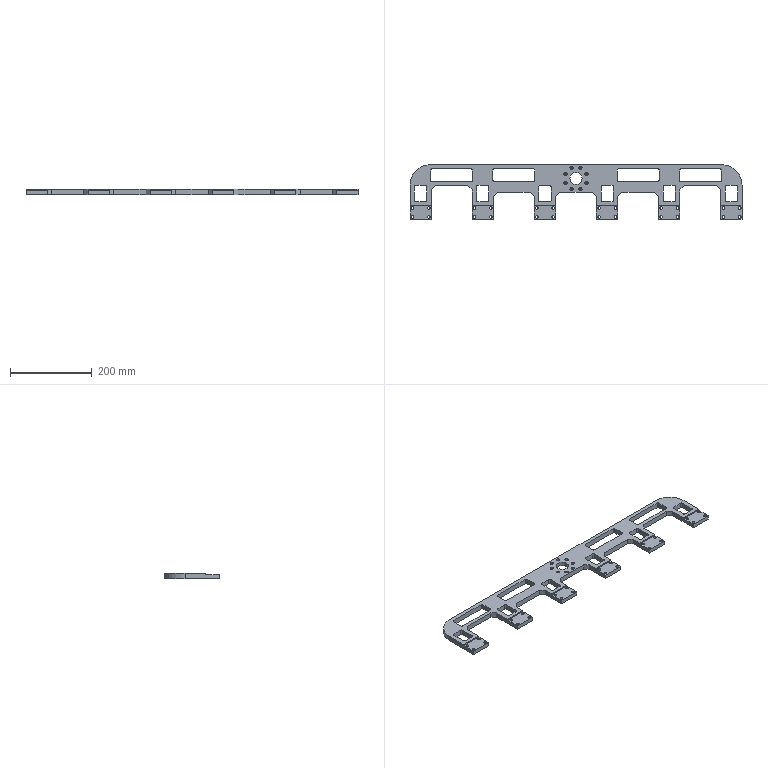NC program | NX | posted with a generic post | part box 813.6 x 134 x 13 mm
Lines 1 to 121 of 6062:
N10 G17 G21 G94 G90
(FLOOR_WALL_COPY_COPY , TOOL : D63)
N12 T01 M6
N14 G54
N16 G17 G0 G90 X-443.3 Y68.997 S6500 M3
N18 G43 Z30. H1
N20 Z3.
N22 G94 G1 Z0. F1500.
N24 X-440.3
N26 X440.3
N28 Y40.798
N30 X-440.3
N32 Y12.599
N34 X440.3
N36 Y-15.601
N38 X-440.3
N40 Y-43.8
N42 X440.3
N44 X443.3
N46 Z3.
N48 G0 Z30.
N50 M5
(DRILLING_COPY_1_COPY , TOOL : D6A45)
N52 T07 M6
N54 G54
N56 G17 G0 G90 X-401.2 Y-61.2 S5000 M3
N58 G43 Z30. H7
N60 G94 G81 G98 Z-1. F250. R3.
N62 Y-39.2
N64 X-361.2
N66 Y-61.2
N68 X-248.8 Y-39.2
N70 Y-61.2
N72 X-208.8
N74 Y-39.2
N76 X-96.4
N78 Y-61.2
N80 X-56.4
N82 Y-39.2
N84 X-10.715 Y7.131
N86 X-25.869 Y22.285
N88 Y43.715
N90 X-10.715 Y58.869
N92 X10.715
N94 X0. Y33.
N96 X25.869 Y43.715
N98 Y22.285
N100 X10.715 Y7.131
N102 X56. Y-39.2
N104 Y-61.2
N106 X96.
N108 Y-39.2
N110 X208.4
N112 Y-61.2
N114 X248.4
N116 Y-39.2
N118 X360.8 Y-61.2
N120 Y-39.2
N122 X400.8
N124 Y-61.2
N126 G80
N128 G0 X400.8 Y-61.2 Z30.
N130 M5
(DRILLING_COPY_COPY_1_COPY , TOOL : 4.5ZT)
N132 T14 M6
N134 G54
N136 G17 G0 G90 X-10.715 Y7.131 S2000 M3
N138 G43 Z30. H14
N140 G94 G83 G98 Z-15.352 F250. Q2. R3.
N142 X10.715
N144 X25.869 Y22.285
N146 Y43.715
N148 X10.715 Y58.869
N150 X-10.715
N152 X-25.869 Y43.715
N154 Y22.285
N156 G80
N158 G0 X-25.869 Y22.285 Z30.
N160 M5
(DRILLING_COPY_COPY_COPY_COPY , TOOL : 6.5ZT)
N162 T15 M6
N164 G54
N166 G17 G0 G90 X400.8 Y-39.2 S2000 M3
N168 G43 Z30. H15
N170 G94 G83 G98 Z-15.953 F250. Q2. R3.
N172 Y-61.2
N174 X360.8
N176 Y-39.2
N178 X248.4
N180 Y-61.2
N182 X208.4
N184 Y-39.2
N186 X96.
N188 Y-61.2
N190 X56.
N192 Y-39.2
N194 X-56.4
N196 Y-61.2
N198 X-96.4
N200 Y-39.2
N202 X-208.8
N204 Y-61.2
N206 X-248.8
N208 Y-39.2
N210 X-361.2
N212 Y-61.2
N214 X-401.2
N216 Y-39.2
N218 G80
N220 G0 X-401.2 Y-39.2 Z30.
N222 M5